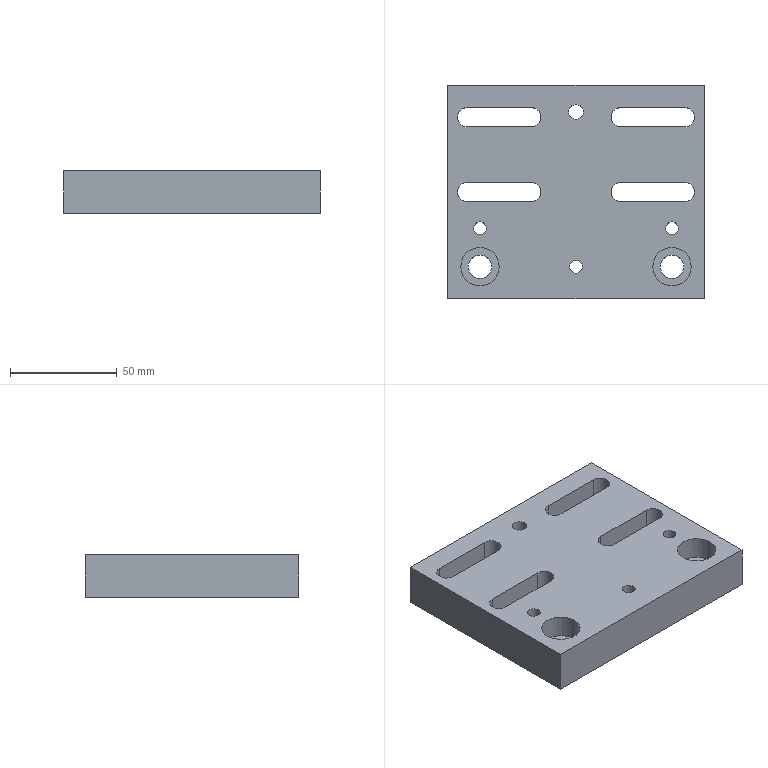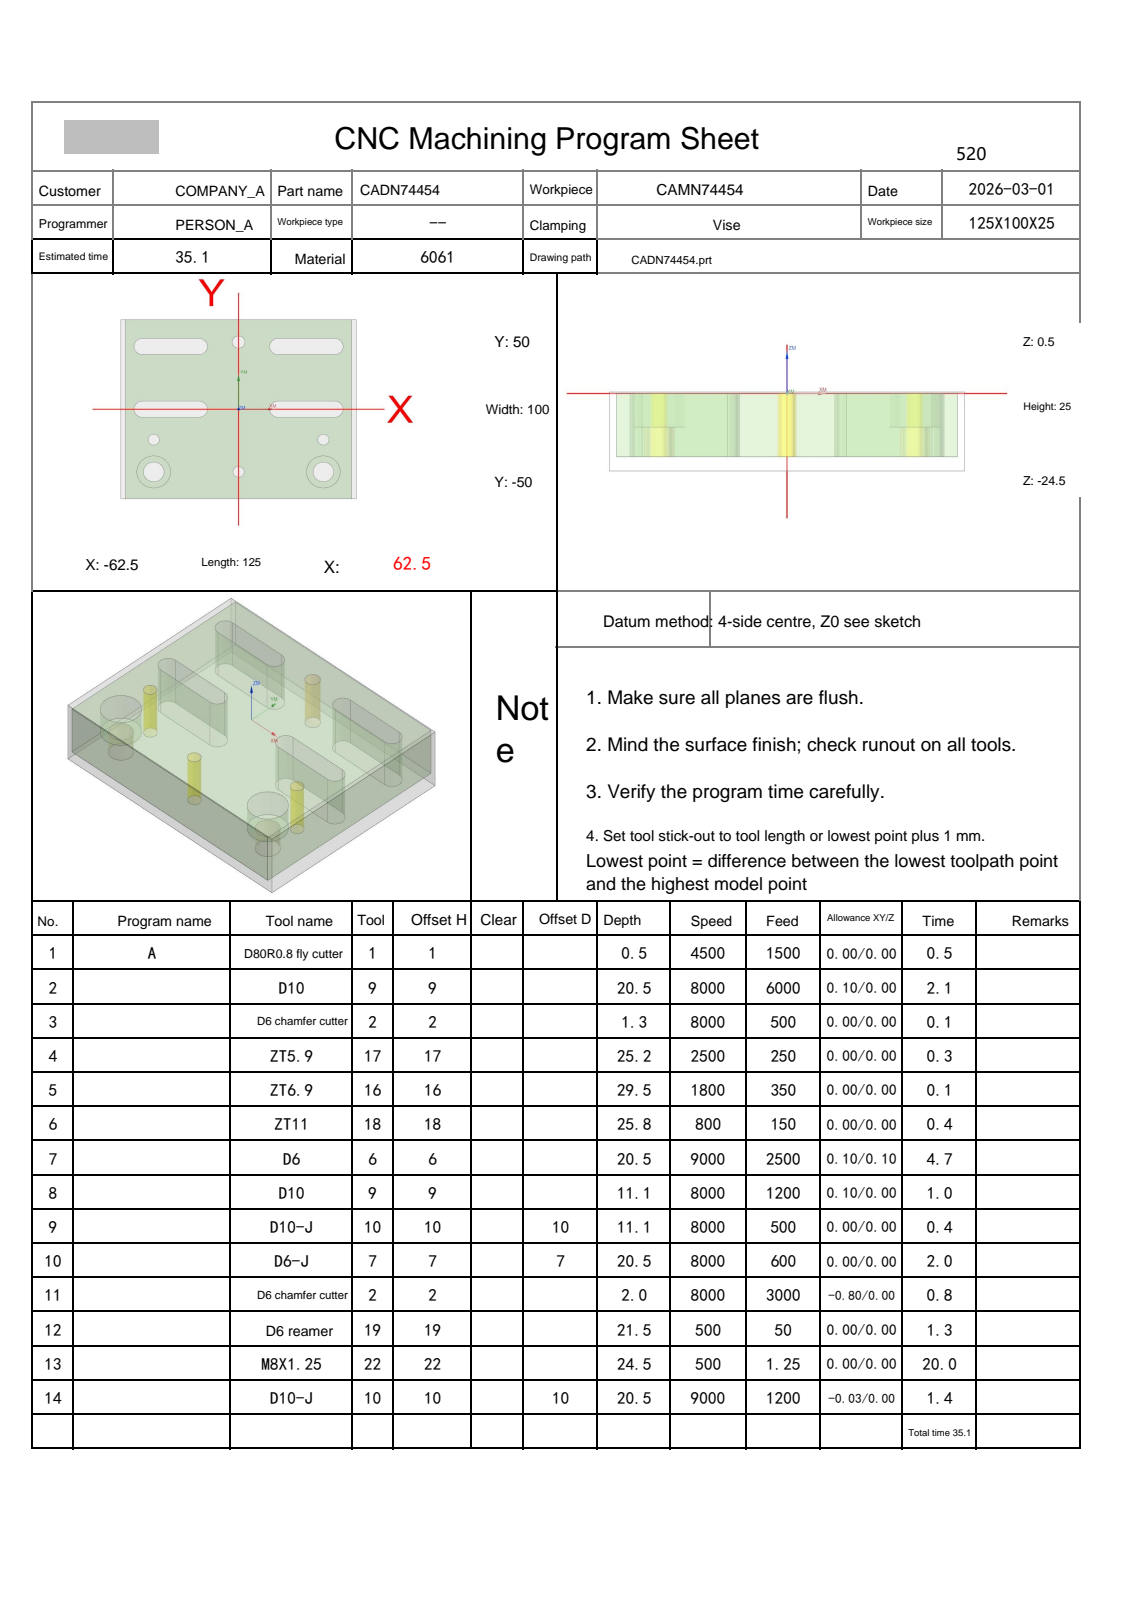NC program | NX | posted by the shop | part box 120 x 100 x 20 mm
Lines 1 to 2069 of 2160, first 1251 of 2067 lines:
%
O0001
(Machine time: 57.03 MIN)
(===Total Tool:11===)
(T1=D80R0.8 fly cutter D=80.  R=0.8  D-  H01 Z=0.    )
(T9=D10     D=10.  R=0.   D-  H09 Z=-20.  )
(T2=D6 chamfer cutter   D=6.   R=0.   D-  H02 Z=-1.5  )
(T17=ZT5.9  D=5.9  DR_a=120 D-  H17 Z=-24.7 )
(T16=ZT6.9  D=6.9  DR_a=120 D-  H16 Z=-29.  )
(T18=ZT11   D=11.  DR_a=118 D-  H18 Z=-25.3 )
(T6=D6      D=6.   R=0.   D-  H06 Z=-20.  )
(T10=D10-J  D=10.  R=0.   D10 H10 Z=-20.  )
(T7=D6-J    D=6.   R=0.   D7  H07 Z=-20.  )
(T19=D6 reamer   D=6.   DR_a=180 D-  H19 Z=-21.  )
(T22=M8X1.25 D=6.8  DR_a=180 D-  H22 Z=-24.  )
G80 G90 G17 G49 G40
G91 G28 Z0
M01
N1 T01 M06
(D80R0.8 fly cutter  D=80. R=0.8 H=01 ce=0.00 di=0.00)
G00 G90 G54 X-105. Y45. M03 S4500
G43 H01 Z50.
M08
Z2.
G01 Z0.0 F1500.
X-100.
X100.
Y0.0
X-100.
Y-45.
X100.
X105.
Z2.
G00 Z50.
G91 G28 Z0.0
M05
M09
G91 G28 Z0.0
M01
N2 T09 M06
(D10  D=10. R=0. H=09 ce=0.10 di=0.00)
G00 G90 G54 X0.0 Y55.1 M03 S8000
G43 H09 Z50.
M08
Z.5
G01 X60. Z.4 F6000.
G02 X65.1 Y50. Z.386 I0.0 J-5.1
G01 Y-50. Z.219
G02 X60. Y-55.1 Z.206 I-5.1 J0.0
G01 X-60. Z.006
G02 X-65.1 Y-50. Z-.008 I0.0 J5.1
G01 Y50. Z-.175
G02 X-60. Y55.1 Z-.188 I5.1 J0.0
G01 X60. Z-.389
G02 X65.1 Y50. Z-.402 I0.0 J-5.1
G01 Y-50. Z-.569
G02 X60. Y-55.1 Z-.582 I-5.1 J0.0
G01 X-60. Z-.783
G02 X-65.1 Y-50. Z-.796 I0.0 J5.1
G01 Y50. Z-.963
G02 X-60. Y55.1 Z-.977 I5.1 J0.0
G01 X60. Z-1.177
G02 X65.1 Y50. Z-1.191 I0.0 J-5.1
G01 Y-50. Z-1.358
G02 X60. Y-55.1 Z-1.371 I-5.1 J0.0
G01 X-60. Z-1.571
G02 X-65.1 Y-50. Z-1.585 I0.0 J5.1
G01 Y50. Z-1.752
G02 X-60. Y55.1 Z-1.765 I5.1 J0.0
G01 X60. Z-1.966
G02 X65.1 Y50. Z-1.979 I0.0 J-5.1
G01 Y-50. Z-2.146
G02 X60. Y-55.1 Z-2.159 I-5.1 J0.0
G01 X-60. Z-2.36
G02 X-65.1 Y-50. Z-2.373 I0.0 J5.1
G01 Y50. Z-2.54
G02 X-60. Y55.1 Z-2.554 I5.1 J0.0
G01 X60. Z-2.754
G02 X65.1 Y50. Z-2.767 I0.0 J-5.1
G01 Y-50. Z-2.934
G02 X60. Y-55.1 Z-2.948 I-5.1 J0.0
G01 X-60. Z-3.148
G02 X-65.1 Y-50. Z-3.162 I0.0 J5.1
G01 Y50. Z-3.329
G02 X-60. Y55.1 Z-3.342 I5.1 J0.0
G01 X60. Z-3.543
G02 X65.1 Y50. Z-3.556 I0.0 J-5.1
G01 Y-50. Z-3.723
G02 X60. Y-55.1 Z-3.736 I-5.1 J0.0
G01 X-60. Z-3.937
G02 X-65.1 Y-50. Z-3.95 I0.0 J5.1
G01 Y50. Z-4.117
G02 X-60. Y55.1 Z-4.131 I5.1 J0.0
G01 X60. Z-4.331
G02 X65.1 Y50. Z-4.344 I0.0 J-5.1
G01 Y-50. Z-4.511
G02 X60. Y-55.1 Z-4.525 I-5.1 J0.0
G01 X-60. Z-4.725
G02 X-65.1 Y-50. Z-4.739 I0.0 J5.1
G01 Y50. Z-4.906
G02 X-60. Y55.1 Z-4.919 I5.1 J0.0
G01 X60. Z-5.119
G02 X65.1 Y50. Z-5.133 I0.0 J-5.1
G01 Y-50. Z-5.3
G02 X60. Y-55.1 Z-5.313 I-5.1 J0.0
G01 X-60. Z-5.514
G02 X-65.1 Y-50. Z-5.527 I0.0 J5.1
G01 Y50. Z-5.694
G02 X-60. Y55.1 Z-5.707 I5.1 J0.0
G01 X60. Z-5.908
G02 X65.1 Y50. Z-5.921 I0.0 J-5.1
G01 Y-50. Z-6.088
G02 X60. Y-55.1 Z-6.102 I-5.1 J0.0
G01 X-60. Z-6.302
G02 X-65.1 Y-50. Z-6.316 I0.0 J5.1
G01 Y50. Z-6.483
G02 X-60. Y55.1 Z-6.496 I5.1 J0.0
G01 X60. Z-6.696
G02 X65.1 Y50. Z-6.71 I0.0 J-5.1
G01 Y-50. Z-6.877
G02 X60. Y-55.1 Z-6.89 I-5.1 J0.0
G01 X-60. Z-7.091
G02 X-65.1 Y-50. Z-7.104 I0.0 J5.1
G01 Y50. Z-7.271
G02 X-60. Y55.1 Z-7.284 I5.1 J0.0
G01 X60. Z-7.485
G02 X65.1 Y50. Z-7.498 I0.0 J-5.1
G01 Y-50. Z-7.665
G02 X60. Y-55.1 Z-7.679 I-5.1 J0.0
G01 X-60. Z-7.879
G02 X-65.1 Y-50. Z-7.892 I0.0 J5.1
G01 Y50. Z-8.059
G02 X-60. Y55.1 Z-8.073 I5.1 J0.0
G01 X60. Z-8.273
G02 X65.1 Y50. Z-8.287 I0.0 J-5.1
G01 Y-50. Z-8.454
G02 X60. Y-55.1 Z-8.467 I-5.1 J0.0
G01 X-60. Z-8.668
G02 X-65.1 Y-50. Z-8.681 I0.0 J5.1
G01 Y50. Z-8.848
G02 X-60. Y55.1 Z-8.861 I5.1 J0.0
G01 X60. Z-9.062
G02 X65.1 Y50. Z-9.075 I0.0 J-5.1
G01 Y-50. Z-9.242
G02 X60. Y-55.1 Z-9.256 I-5.1 J0.0
G01 X-60. Z-9.456
G02 X-65.1 Y-50. Z-9.469 I0.0 J5.1
G01 Y50. Z-9.636
G02 X-60. Y55.1 Z-9.65 I5.1 J0.0
G01 X60. Z-9.85
G02 X65.1 Y50. Z-9.864 I0.0 J-5.1
G01 Y-50. Z-10.031
G02 X60. Y-55.1 Z-10.044 I-5.1 J0.0
G01 X-60. Z-10.244
G02 X-65.1 Y-50. Z-10.258 I0.0 J5.1
G01 Y50. Z-10.425
G02 X-60. Y55.1 Z-10.438 I5.1 J0.0
G01 X60. Z-10.639
G02 X65.1 Y50. Z-10.652 I0.0 J-5.1
G01 Y-50. Z-10.819
G02 X60. Y-55.1 Z-10.832 I-5.1 J0.0
G01 X-60. Z-11.033
G02 X-65.1 Y-50. Z-11.046 I0.0 J5.1
G01 Y50. Z-11.213
G02 X-60. Y55.1 Z-11.227 I5.1 J0.0
G01 X60. Z-11.427
G02 X65.1 Y50. Z-11.441 I0.0 J-5.1
G01 Y-50. Z-11.608
G02 X60. Y-55.1 Z-11.621 I-5.1 J0.0
G01 X-60. Z-11.821
G02 X-65.1 Y-50. Z-11.835 I0.0 J5.1
G01 Y50. Z-12.002
G02 X-60. Y55.1 Z-12.015 I5.1 J0.0
G01 X60. Z-12.216
G02 X65.1 Y50. Z-12.229 I0.0 J-5.1
G01 Y-50. Z-12.396
G02 X60. Y-55.1 Z-12.409 I-5.1 J0.0
G01 X-60. Z-12.61
G02 X-65.1 Y-50. Z-12.623 I0.0 J5.1
G01 Y50. Z-12.79
G02 X-60. Y55.1 Z-12.804 I5.1 J0.0
G01 X60. Z-13.004
G02 X65.1 Y50. Z-13.017 I0.0 J-5.1
G01 Y-50. Z-13.184
G02 X60. Y-55.1 Z-13.198 I-5.1 J0.0
G01 X-60. Z-13.398
G02 X-65.1 Y-50. Z-13.412 I0.0 J5.1
G01 Y50. Z-13.579
G02 X-60. Y55.1 Z-13.592 I5.1 J0.0
G01 X60. Z-13.793
G02 X65.1 Y50. Z-13.806 I0.0 J-5.1
G01 Y-50. Z-13.973
G02 X60. Y-55.1 Z-13.986 I-5.1 J0.0
G01 X-60. Z-14.187
G02 X-65.1 Y-50. Z-14.2 I0.0 J5.1
G01 Y50. Z-14.367
G02 X-60. Y55.1 Z-14.381 I5.1 J0.0
G01 X60. Z-14.581
G02 X65.1 Y50. Z-14.594 I0.0 J-5.1
G01 Y-50. Z-14.761
G02 X60. Y-55.1 Z-14.775 I-5.1 J0.0
G01 X-60. Z-14.975
G02 X-65.1 Y-50. Z-14.989 I0.0 J5.1
G01 Y50. Z-15.156
G02 X-60. Y55.1 Z-15.169 I5.1 J0.0
G01 X60. Z-15.369
G02 X65.1 Y50. Z-15.383 I0.0 J-5.1
G01 Y-50. Z-15.55
G02 X60. Y-55.1 Z-15.563 I-5.1 J0.0
G01 X-60. Z-15.764
G02 X-65.1 Y-50. Z-15.777 I0.0 J5.1
G01 Y50. Z-15.944
G02 X-60. Y55.1 Z-15.957 I5.1 J0.0
G01 X60. Z-16.158
G02 X65.1 Y50. Z-16.171 I0.0 J-5.1
G01 Y-50. Z-16.338
G02 X60. Y-55.1 Z-16.352 I-5.1 J0.0
G01 X-60. Z-16.552
G02 X-65.1 Y-50. Z-16.566 I0.0 J5.1
G01 Y50. Z-16.733
G02 X-60. Y55.1 Z-16.746 I5.1 J0.0
G01 X60. Z-16.946
G02 X65.1 Y50. Z-16.96 I0.0 J-5.1
G01 Y-50. Z-17.127
G02 X60. Y-55.1 Z-17.14 I-5.1 J0.0
G01 X-60. Z-17.341
G02 X-65.1 Y-50. Z-17.354 I0.0 J5.1
G01 Y50. Z-17.521
G02 X-60. Y55.1 Z-17.534 I5.1 J0.0
G01 X60. Z-17.735
G02 X65.1 Y50. Z-17.748 I0.0 J-5.1
G01 Y-50. Z-17.915
G02 X60. Y-55.1 Z-17.929 I-5.1 J0.0
G01 X-60. Z-18.129
G02 X-65.1 Y-50. Z-18.142 I0.0 J5.1
G01 Y50. Z-18.309
G02 X-60. Y55.1 Z-18.323 I5.1 J0.0
G01 X60. Z-18.523
G02 X65.1 Y50. Z-18.537 I0.0 J-5.1
G01 Y-50. Z-18.704
G02 X60. Y-55.1 Z-18.717 I-5.1 J0.0
G01 X-60. Z-18.918
G02 X-65.1 Y-50. Z-18.931 I0.0 J5.1
G01 Y50. Z-19.098
G02 X-60. Y55.1 Z-19.111 I5.1 J0.0
G01 X60. Z-19.312
G02 X65.1 Y50. Z-19.325 I0.0 J-5.1
G01 Y-50. Z-19.492
G02 X60. Y-55.1 Z-19.506 I-5.1 J0.0
G01 X-60. Z-19.706
G02 X-65.1 Y-50. Z-19.719 I0.0 J5.1
G01 Y50. Z-19.886
G02 X-60. Y55.1 Z-19.9 I5.1 J0.0
G01 X0.0 Z-20.
X60.
G02 X65.1 Y50. I0.0 J-5.1
G01 Y-50.
G02 X60. Y-55.1 I-5.1 J0.0
G01 X-60.
G02 X-65.1 Y-50. I0.0 J5.1
G01 Y50.
G02 X-60. Y55.1 I5.1 J0.0
G01 X0.0
X.5
Z-19.
G00 Z50.
G91 G28 Z0.0
M05
M09
G91 G28 Z0.0
M01
N3 T02 M06
(D6 chamfer cutter  D=6. R=0. H=02 ce=0.00 di=0.00)
G00 G90 G54 X45. Y-17. M03 S8000
G43 H02 Z50.
M08
G98 G81 X45. Y-17. Z-.8 R1. F500.
Y-35.
X0.0
X-45.
Y-17.
X0.0 Y37.5
G80
G00 Z50.
G91 G28 Z0.0
M05
M09
G91 G28 Z0.0
M01
N4 T17 M06
(ZT5.9 D=5.9 DR_a=120 H=17)
G00 G90 G54 X45. Y-17. M03 S2500
G43 H17 Z50.
M08
G98 G83 X45. Y-17. Z-24.703 R1. F250. Q2.
X0.0 Y-35.
X-45. Y-17.
G80
G00 Z50.
G91 G28 Z0.0
M05
M09
G91 G28 Z0.0
M01
N5 T16 M06
(ZT6.9 D=6.9 DR_a=120 H=16)
G00 G90 G54 X0.0 Y37.5 M03 S1800
G43 H16 Z50.
M08
G98 G83 X0.0 Y37.5 Z-29. R1. F350. Q3.
G80
G00 Z50.
G91 G28 Z0.0
M05
M09
G91 G28 Z0.0
M01
N6 T18 M06
(ZT11 D=11. DR_a=118 H=18)
G00 G90 G54 X-45. Y-35. M03 S800
G43 H18 Z50.
M08
G98 G83 X-45. Y-35. Z-25.305 R1. F150. Q2.
X45.
G80
G00 Z50.
G91 G28 Z0.0
M05
M09
G91 G28 Z0.0
M01
N7 T06 M06
(D6  D=6. R=0. H=06 ce=0.10 di=0.10)
G00 G90 G54 X36. Y36.4 M03 S9000
G43 H06 Z50.
M08
Z.5
G01 X21. Z.391 F2500.
G03 X19.6 Y35. Z.375 I0.0 J-1.4
X21. Y33.6 Z.359 I1.4 J0.0
G01 X51. Z.141
G03 X52.4 Y35. Z.125 I0.0 J1.4
X51. Y36.4 Z.109 I-1.4 J0.0
G01 X21. Z-.109
G03 X19.6 Y35. Z-.125 I0.0 J-1.4
X21. Y33.6 Z-.141 I1.4 J0.0
G01 X51. Z-.359
G03 X52.4 Y35. Z-.375 I0.0 J1.4
X51. Y36.4 Z-.391 I-1.4 J0.0
G01 X21. Z-.609
G03 X19.6 Y35. Z-.625 I0.0 J-1.4
X21. Y33.6 Z-.641 I1.4 J0.0
G01 X51. Z-.859
G03 X52.4 Y35. Z-.875 I0.0 J1.4
X51. Y36.4 Z-.891 I-1.4 J0.0
G01 X21. Z-1.109
G03 X19.6 Y35. Z-1.125 I0.0 J-1.4
X21. Y33.6 Z-1.141 I1.4 J0.0
G01 X51. Z-1.359
G03 X52.4 Y35. Z-1.375 I0.0 J1.4
X51. Y36.4 Z-1.391 I-1.4 J0.0
G01 X21. Z-1.609
G03 X19.6 Y35. Z-1.625 I0.0 J-1.4
X21. Y33.6 Z-1.641 I1.4 J0.0
G01 X51. Z-1.859
G03 X52.4 Y35. Z-1.875 I0.0 J1.4
X51. Y36.4 Z-1.891 I-1.4 J0.0
G01 X21. Z-2.109
G03 X19.6 Y35. Z-2.125 I0.0 J-1.4
X21. Y33.6 Z-2.141 I1.4 J0.0
G01 X51. Z-2.359
G03 X52.4 Y35. Z-2.375 I0.0 J1.4
X51. Y36.4 Z-2.391 I-1.4 J0.0
G01 X21. Z-2.609
G03 X19.6 Y35. Z-2.625 I0.0 J-1.4
X21. Y33.6 Z-2.641 I1.4 J0.0
G01 X51. Z-2.859
G03 X52.4 Y35. Z-2.875 I0.0 J1.4
X51. Y36.4 Z-2.891 I-1.4 J0.0
G01 X21. Z-3.109
G03 X19.6 Y35. Z-3.125 I0.0 J-1.4
X21. Y33.6 Z-3.141 I1.4 J0.0
G01 X51. Z-3.359
G03 X52.4 Y35. Z-3.375 I0.0 J1.4
X51. Y36.4 Z-3.391 I-1.4 J0.0
G01 X21. Z-3.609
G03 X19.6 Y35. Z-3.625 I0.0 J-1.4
X21. Y33.6 Z-3.641 I1.4 J0.0
G01 X51. Z-3.859
G03 X52.4 Y35. Z-3.875 I0.0 J1.4
X51. Y36.4 Z-3.891 I-1.4 J0.0
G01 X21. Z-4.109
G03 X19.6 Y35. Z-4.125 I0.0 J-1.4
X21. Y33.6 Z-4.141 I1.4 J0.0
G01 X51. Z-4.359
G03 X52.4 Y35. Z-4.375 I0.0 J1.4
X51. Y36.4 Z-4.391 I-1.4 J0.0
G01 X21. Z-4.609
G03 X19.6 Y35. Z-4.625 I0.0 J-1.4
X21. Y33.6 Z-4.641 I1.4 J0.0
G01 X51. Z-4.859
G03 X52.4 Y35. Z-4.875 I0.0 J1.4
X51. Y36.4 Z-4.891 I-1.4 J0.0
G01 X21. Z-5.109
G03 X19.6 Y35. Z-5.125 I0.0 J-1.4
X21. Y33.6 Z-5.141 I1.4 J0.0
G01 X51. Z-5.359
G03 X52.4 Y35. Z-5.375 I0.0 J1.4
X51. Y36.4 Z-5.391 I-1.4 J0.0
G01 X21. Z-5.609
G03 X19.6 Y35. Z-5.625 I0.0 J-1.4
X21. Y33.6 Z-5.641 I1.4 J0.0
G01 X51. Z-5.859
G03 X52.4 Y35. Z-5.875 I0.0 J1.4
X51. Y36.4 Z-5.891 I-1.4 J0.0
G01 X21. Z-6.109
G03 X19.6 Y35. Z-6.125 I0.0 J-1.4
X21. Y33.6 Z-6.141 I1.4 J0.0
G01 X51. Z-6.359
G03 X52.4 Y35. Z-6.375 I0.0 J1.4
X51. Y36.4 Z-6.391 I-1.4 J0.0
G01 X21. Z-6.609
G03 X19.6 Y35. Z-6.625 I0.0 J-1.4
X21. Y33.6 Z-6.641 I1.4 J0.0
G01 X51. Z-6.859
G03 X52.4 Y35. Z-6.875 I0.0 J1.4
X51. Y36.4 Z-6.891 I-1.4 J0.0
G01 X21. Z-7.109
G03 X19.6 Y35. Z-7.125 I0.0 J-1.4
X21. Y33.6 Z-7.141 I1.4 J0.0
G01 X51. Z-7.359
G03 X52.4 Y35. Z-7.375 I0.0 J1.4
X51. Y36.4 Z-7.391 I-1.4 J0.0
G01 X21. Z-7.609
G03 X19.6 Y35. Z-7.625 I0.0 J-1.4
X21. Y33.6 Z-7.641 I1.4 J0.0
G01 X51. Z-7.859
G03 X52.4 Y35. Z-7.875 I0.0 J1.4
X51. Y36.4 Z-7.891 I-1.4 J0.0
G01 X21. Z-8.109
G03 X19.6 Y35. Z-8.125 I0.0 J-1.4
X21. Y33.6 Z-8.141 I1.4 J0.0
G01 X51. Z-8.359
G03 X52.4 Y35. Z-8.375 I0.0 J1.4
X51. Y36.4 Z-8.391 I-1.4 J0.0
G01 X21. Z-8.609
G03 X19.6 Y35. Z-8.625 I0.0 J-1.4
X21. Y33.6 Z-8.641 I1.4 J0.0
G01 X51. Z-8.859
G03 X52.4 Y35. Z-8.875 I0.0 J1.4
X51. Y36.4 Z-8.891 I-1.4 J0.0
G01 X21. Z-9.109
G03 X19.6 Y35. Z-9.125 I0.0 J-1.4
X21. Y33.6 Z-9.141 I1.4 J0.0
G01 X51. Z-9.359
G03 X52.4 Y35. Z-9.375 I0.0 J1.4
X51. Y36.4 Z-9.391 I-1.4 J0.0
G01 X21. Z-9.609
G03 X19.6 Y35. Z-9.625 I0.0 J-1.4
X21. Y33.6 Z-9.641 I1.4 J0.0
G01 X51. Z-9.859
G03 X52.4 Y35. Z-9.875 I0.0 J1.4
X51. Y36.4 Z-9.891 I-1.4 J0.0
G01 X21. Z-10.109
G03 X19.6 Y35. Z-10.125 I0.0 J-1.4
X21. Y33.6 Z-10.141 I1.4 J0.0
G01 X51. Z-10.359
G03 X52.4 Y35. Z-10.375 I0.0 J1.4
X51. Y36.4 Z-10.391 I-1.4 J0.0
G01 X21. Z-10.609
G03 X19.6 Y35. Z-10.625 I0.0 J-1.4
X21. Y33.6 Z-10.641 I1.4 J0.0
G01 X51. Z-10.859
G03 X52.4 Y35. Z-10.875 I0.0 J1.4
X51. Y36.4 Z-10.891 I-1.4 J0.0
G01 X21. Z-11.109
G03 X19.6 Y35. Z-11.125 I0.0 J-1.4
X21. Y33.6 Z-11.141 I1.4 J0.0
G01 X51. Z-11.359
G03 X52.4 Y35. Z-11.375 I0.0 J1.4
X51. Y36.4 Z-11.391 I-1.4 J0.0
G01 X21. Z-11.609
G03 X19.6 Y35. Z-11.625 I0.0 J-1.4
X21. Y33.6 Z-11.641 I1.4 J0.0
G01 X51. Z-11.859
G03 X52.4 Y35. Z-11.875 I0.0 J1.4
X51. Y36.4 Z-11.891 I-1.4 J0.0
G01 X21. Z-12.109
G03 X19.6 Y35. Z-12.125 I0.0 J-1.4
X21. Y33.6 Z-12.141 I1.4 J0.0
G01 X51. Z-12.359
G03 X52.4 Y35. Z-12.375 I0.0 J1.4
X51. Y36.4 Z-12.391 I-1.4 J0.0
G01 X21. Z-12.609
G03 X19.6 Y35. Z-12.625 I0.0 J-1.4
X21. Y33.6 Z-12.641 I1.4 J0.0
G01 X51. Z-12.859
G03 X52.4 Y35. Z-12.875 I0.0 J1.4
X51. Y36.4 Z-12.891 I-1.4 J0.0
G01 X21. Z-13.109
G03 X19.6 Y35. Z-13.125 I0.0 J-1.4
X21. Y33.6 Z-13.141 I1.4 J0.0
G01 X51. Z-13.359
G03 X52.4 Y35. Z-13.375 I0.0 J1.4
X51. Y36.4 Z-13.391 I-1.4 J0.0
G01 X21. Z-13.609
G03 X19.6 Y35. Z-13.625 I0.0 J-1.4
X21. Y33.6 Z-13.641 I1.4 J0.0
G01 X51. Z-13.859
G03 X52.4 Y35. Z-13.875 I0.0 J1.4
X51. Y36.4 Z-13.891 I-1.4 J0.0
G01 X21. Z-14.109
G03 X19.6 Y35. Z-14.125 I0.0 J-1.4
X21. Y33.6 Z-14.141 I1.4 J0.0
G01 X51. Z-14.359
G03 X52.4 Y35. Z-14.375 I0.0 J1.4
X51. Y36.4 Z-14.391 I-1.4 J0.0
G01 X21. Z-14.609
G03 X19.6 Y35. Z-14.625 I0.0 J-1.4
X21. Y33.6 Z-14.641 I1.4 J0.0
G01 X51. Z-14.859
G03 X52.4 Y35. Z-14.875 I0.0 J1.4
X51. Y36.4 Z-14.891 I-1.4 J0.0
G01 X21. Z-15.109
G03 X19.6 Y35. Z-15.125 I0.0 J-1.4
X21. Y33.6 Z-15.141 I1.4 J0.0
G01 X51. Z-15.359
G03 X52.4 Y35. Z-15.375 I0.0 J1.4
X51. Y36.4 Z-15.391 I-1.4 J0.0
G01 X21. Z-15.609
G03 X19.6 Y35. Z-15.625 I0.0 J-1.4
X21. Y33.6 Z-15.641 I1.4 J0.0
G01 X51. Z-15.859
G03 X52.4 Y35. Z-15.875 I0.0 J1.4
X51. Y36.4 Z-15.891 I-1.4 J0.0
G01 X21. Z-16.109
G03 X19.6 Y35. Z-16.125 I0.0 J-1.4
X21. Y33.6 Z-16.141 I1.4 J0.0
G01 X51. Z-16.359
G03 X52.4 Y35. Z-16.375 I0.0 J1.4
X51. Y36.4 Z-16.391 I-1.4 J0.0
G01 X21. Z-16.609
G03 X19.6 Y35. Z-16.625 I0.0 J-1.4
X21. Y33.6 Z-16.641 I1.4 J0.0
G01 X51. Z-16.859
G03 X52.4 Y35. Z-16.875 I0.0 J1.4
X51. Y36.4 Z-16.891 I-1.4 J0.0
G01 X21. Z-17.109
G03 X19.6 Y35. Z-17.125 I0.0 J-1.4
X21. Y33.6 Z-17.141 I1.4 J0.0
G01 X51. Z-17.359
G03 X52.4 Y35. Z-17.375 I0.0 J1.4
X51. Y36.4 Z-17.391 I-1.4 J0.0
G01 X21. Z-17.609
G03 X19.6 Y35. Z-17.625 I0.0 J-1.4
X21. Y33.6 Z-17.641 I1.4 J0.0
G01 X51. Z-17.859
G03 X52.4 Y35. Z-17.875 I0.0 J1.4
X51. Y36.4 Z-17.891 I-1.4 J0.0
G01 X21. Z-18.109
G03 X19.6 Y35. Z-18.125 I0.0 J-1.4
X21. Y33.6 Z-18.141 I1.4 J0.0
G01 X51. Z-18.359
G03 X52.4 Y35. Z-18.375 I0.0 J1.4
X51. Y36.4 Z-18.391 I-1.4 J0.0
G01 X21. Z-18.609
G03 X19.6 Y35. Z-18.625 I0.0 J-1.4
X21. Y33.6 Z-18.641 I1.4 J0.0
G01 X51. Z-18.859
G03 X52.4 Y35. Z-18.875 I0.0 J1.4
X51. Y36.4 Z-18.891 I-1.4 J0.0
G01 X21. Z-19.109
G03 X19.6 Y35. Z-19.125 I0.0 J-1.4
X21. Y33.6 Z-19.141 I1.4 J0.0
G01 X51. Z-19.359
G03 X52.4 Y35. Z-19.375 I0.0 J1.4
X51. Y36.4 Z-19.391 I-1.4 J0.0
G01 X21. Z-19.609
G03 X19.6 Y35. Z-19.625 I0.0 J-1.4
X21. Y33.6 Z-19.641 I1.4 J0.0
G01 X51. Z-19.859
G03 X52.4 Y35. Z-19.875 I0.0 J1.4
X51. Y36.4 Z-19.891 I-1.4 J0.0
G01 X36. Z-20.
X21.
G03 X19.6 Y35. I0.0 J-1.4
X21. Y33.6 I1.4 J0.0
G01 X51.
G03 X52.4 Y35. I0.0 J1.4
X51. Y36.4 I-1.4 J0.0
G01 X36.
X35.5
Z-19.
G00 Z50.
X36. Y1.4
Z.5
G01 X21. Z.391
G03 X19.6 Y0.0 Z.375 I0.0 J-1.4
X21. Y-1.4 Z.359 I1.4 J0.0
G01 X51. Z.141
G03 X52.4 Y0.0 Z.125 I0.0 J1.4
X51. Y1.4 Z.109 I-1.4 J0.0
G01 X21. Z-.109
G03 X19.6 Y0.0 Z-.125 I0.0 J-1.4
X21. Y-1.4 Z-.141 I1.4 J0.0
G01 X51. Z-.359
G03 X52.4 Y0.0 Z-.375 I0.0 J1.4
X51. Y1.4 Z-.391 I-1.4 J0.0
G01 X21. Z-.609
G03 X19.6 Y0.0 Z-.625 I0.0 J-1.4
X21. Y-1.4 Z-.641 I1.4 J0.0
G01 X51. Z-.859
G03 X52.4 Y0.0 Z-.875 I0.0 J1.4
X51. Y1.4 Z-.891 I-1.4 J0.0
G01 X21. Z-1.109
G03 X19.6 Y0.0 Z-1.125 I0.0 J-1.4
X21. Y-1.4 Z-1.141 I1.4 J0.0
G01 X51. Z-1.359
G03 X52.4 Y0.0 Z-1.375 I0.0 J1.4
X51. Y1.4 Z-1.391 I-1.4 J0.0
G01 X21. Z-1.609
G03 X19.6 Y0.0 Z-1.625 I0.0 J-1.4
X21. Y-1.4 Z-1.641 I1.4 J0.0
G01 X51. Z-1.859
G03 X52.4 Y0.0 Z-1.875 I0.0 J1.4
X51. Y1.4 Z-1.891 I-1.4 J0.0
G01 X21. Z-2.109
G03 X19.6 Y0.0 Z-2.125 I0.0 J-1.4
X21. Y-1.4 Z-2.141 I1.4 J0.0
G01 X51. Z-2.359
G03 X52.4 Y0.0 Z-2.375 I0.0 J1.4
X51. Y1.4 Z-2.391 I-1.4 J0.0
G01 X21. Z-2.609
G03 X19.6 Y0.0 Z-2.625 I0.0 J-1.4
X21. Y-1.4 Z-2.641 I1.4 J0.0
G01 X51. Z-2.859
G03 X52.4 Y0.0 Z-2.875 I0.0 J1.4
X51. Y1.4 Z-2.891 I-1.4 J0.0
G01 X21. Z-3.109
G03 X19.6 Y0.0 Z-3.125 I0.0 J-1.4
X21. Y-1.4 Z-3.141 I1.4 J0.0
G01 X51. Z-3.359
G03 X52.4 Y0.0 Z-3.375 I0.0 J1.4
X51. Y1.4 Z-3.391 I-1.4 J0.0
G01 X21. Z-3.609
G03 X19.6 Y0.0 Z-3.625 I0.0 J-1.4
X21. Y-1.4 Z-3.641 I1.4 J0.0
G01 X51. Z-3.859
G03 X52.4 Y0.0 Z-3.875 I0.0 J1.4
X51. Y1.4 Z-3.891 I-1.4 J0.0
G01 X21. Z-4.109
G03 X19.6 Y0.0 Z-4.125 I0.0 J-1.4
X21. Y-1.4 Z-4.141 I1.4 J0.0
G01 X51. Z-4.359
G03 X52.4 Y0.0 Z-4.375 I0.0 J1.4
X51. Y1.4 Z-4.391 I-1.4 J0.0
G01 X21. Z-4.609
G03 X19.6 Y0.0 Z-4.625 I0.0 J-1.4
X21. Y-1.4 Z-4.641 I1.4 J0.0
G01 X51. Z-4.859
G03 X52.4 Y0.0 Z-4.875 I0.0 J1.4
X51. Y1.4 Z-4.891 I-1.4 J0.0
G01 X21. Z-5.109
G03 X19.6 Y0.0 Z-5.125 I0.0 J-1.4
X21. Y-1.4 Z-5.141 I1.4 J0.0
G01 X51. Z-5.359
G03 X52.4 Y0.0 Z-5.375 I0.0 J1.4
X51. Y1.4 Z-5.391 I-1.4 J0.0
G01 X21. Z-5.609
G03 X19.6 Y0.0 Z-5.625 I0.0 J-1.4
X21. Y-1.4 Z-5.641 I1.4 J0.0
G01 X51. Z-5.859
G03 X52.4 Y0.0 Z-5.875 I0.0 J1.4
X51. Y1.4 Z-5.891 I-1.4 J0.0
G01 X21. Z-6.109
G03 X19.6 Y0.0 Z-6.125 I0.0 J-1.4
X21. Y-1.4 Z-6.141 I1.4 J0.0
G01 X51. Z-6.359
G03 X52.4 Y0.0 Z-6.375 I0.0 J1.4
X51. Y1.4 Z-6.391 I-1.4 J0.0
G01 X21. Z-6.609
G03 X19.6 Y0.0 Z-6.625 I0.0 J-1.4
X21. Y-1.4 Z-6.641 I1.4 J0.0
G01 X51. Z-6.859
G03 X52.4 Y0.0 Z-6.875 I0.0 J1.4
X51. Y1.4 Z-6.891 I-1.4 J0.0
G01 X21. Z-7.109
G03 X19.6 Y0.0 Z-7.125 I0.0 J-1.4
X21. Y-1.4 Z-7.141 I1.4 J0.0
G01 X51. Z-7.359
G03 X52.4 Y0.0 Z-7.375 I0.0 J1.4
X51. Y1.4 Z-7.391 I-1.4 J0.0
G01 X21. Z-7.609
G03 X19.6 Y0.0 Z-7.625 I0.0 J-1.4
X21. Y-1.4 Z-7.641 I1.4 J0.0
G01 X51. Z-7.859
G03 X52.4 Y0.0 Z-7.875 I0.0 J1.4
X51. Y1.4 Z-7.891 I-1.4 J0.0
G01 X21. Z-8.109
G03 X19.6 Y0.0 Z-8.125 I0.0 J-1.4
X21. Y-1.4 Z-8.141 I1.4 J0.0
G01 X51. Z-8.359
G03 X52.4 Y0.0 Z-8.375 I0.0 J1.4
X51. Y1.4 Z-8.391 I-1.4 J0.0
G01 X21. Z-8.609
G03 X19.6 Y0.0 Z-8.625 I0.0 J-1.4
X21. Y-1.4 Z-8.641 I1.4 J0.0
G01 X51. Z-8.859
G03 X52.4 Y0.0 Z-8.875 I0.0 J1.4
X51. Y1.4 Z-8.891 I-1.4 J0.0
G01 X21. Z-9.109
G03 X19.6 Y0.0 Z-9.125 I0.0 J-1.4
X21. Y-1.4 Z-9.141 I1.4 J0.0
G01 X51. Z-9.359
G03 X52.4 Y0.0 Z-9.375 I0.0 J1.4
X51. Y1.4 Z-9.391 I-1.4 J0.0
G01 X21. Z-9.609
G03 X19.6 Y0.0 Z-9.625 I0.0 J-1.4
X21. Y-1.4 Z-9.641 I1.4 J0.0
G01 X51. Z-9.859
G03 X52.4 Y0.0 Z-9.875 I0.0 J1.4
X51. Y1.4 Z-9.891 I-1.4 J0.0
G01 X21. Z-10.109
G03 X19.6 Y0.0 Z-10.125 I0.0 J-1.4
X21. Y-1.4 Z-10.141 I1.4 J0.0
G01 X51. Z-10.359
G03 X52.4 Y0.0 Z-10.375 I0.0 J1.4
X51. Y1.4 Z-10.391 I-1.4 J0.0
G01 X21. Z-10.609
G03 X19.6 Y0.0 Z-10.625 I0.0 J-1.4
X21. Y-1.4 Z-10.641 I1.4 J0.0
G01 X51. Z-10.859
G03 X52.4 Y0.0 Z-10.875 I0.0 J1.4
X51. Y1.4 Z-10.891 I-1.4 J0.0
G01 X21. Z-11.109
G03 X19.6 Y0.0 Z-11.125 I0.0 J-1.4
X21. Y-1.4 Z-11.141 I1.4 J0.0
G01 X51. Z-11.359
G03 X52.4 Y0.0 Z-11.375 I0.0 J1.4
X51. Y1.4 Z-11.391 I-1.4 J0.0
G01 X21. Z-11.609
G03 X19.6 Y0.0 Z-11.625 I0.0 J-1.4
X21. Y-1.4 Z-11.641 I1.4 J0.0
G01 X51. Z-11.859
G03 X52.4 Y0.0 Z-11.875 I0.0 J1.4
X51. Y1.4 Z-11.891 I-1.4 J0.0
G01 X21. Z-12.109
G03 X19.6 Y0.0 Z-12.125 I0.0 J-1.4
X21. Y-1.4 Z-12.141 I1.4 J0.0
G01 X51. Z-12.359
G03 X52.4 Y0.0 Z-12.375 I0.0 J1.4
X51. Y1.4 Z-12.391 I-1.4 J0.0
G01 X21. Z-12.609
G03 X19.6 Y0.0 Z-12.625 I0.0 J-1.4
X21. Y-1.4 Z-12.641 I1.4 J0.0
G01 X51. Z-12.859
G03 X52.4 Y0.0 Z-12.875 I0.0 J1.4
X51. Y1.4 Z-12.891 I-1.4 J0.0
G01 X21. Z-13.109
G03 X19.6 Y0.0 Z-13.125 I0.0 J-1.4
X21. Y-1.4 Z-13.141 I1.4 J0.0
G01 X51. Z-13.359
G03 X52.4 Y0.0 Z-13.375 I0.0 J1.4
X51. Y1.4 Z-13.391 I-1.4 J0.0
G01 X21. Z-13.609
G03 X19.6 Y0.0 Z-13.625 I0.0 J-1.4
X21. Y-1.4 Z-13.641 I1.4 J0.0
G01 X51. Z-13.859
G03 X52.4 Y0.0 Z-13.875 I0.0 J1.4
X51. Y1.4 Z-13.891 I-1.4 J0.0
G01 X21. Z-14.109
G03 X19.6 Y0.0 Z-14.125 I0.0 J-1.4
X21. Y-1.4 Z-14.141 I1.4 J0.0
G01 X51. Z-14.359
G03 X52.4 Y0.0 Z-14.375 I0.0 J1.4
X51. Y1.4 Z-14.391 I-1.4 J0.0
G01 X21. Z-14.609
G03 X19.6 Y0.0 Z-14.625 I0.0 J-1.4
X21. Y-1.4 Z-14.641 I1.4 J0.0
G01 X51. Z-14.859
G03 X52.4 Y0.0 Z-14.875 I0.0 J1.4
X51. Y1.4 Z-14.891 I-1.4 J0.0
G01 X21. Z-15.109
G03 X19.6 Y0.0 Z-15.125 I0.0 J-1.4
X21. Y-1.4 Z-15.141 I1.4 J0.0
G01 X51. Z-15.359
G03 X52.4 Y0.0 Z-15.375 I0.0 J1.4
X51. Y1.4 Z-15.391 I-1.4 J0.0
G01 X21. Z-15.609
G03 X19.6 Y0.0 Z-15.625 I0.0 J-1.4
X21. Y-1.4 Z-15.641 I1.4 J0.0
G01 X51. Z-15.859
G03 X52.4 Y0.0 Z-15.875 I0.0 J1.4
X51. Y1.4 Z-15.891 I-1.4 J0.0
G01 X21. Z-16.109
G03 X19.6 Y0.0 Z-16.125 I0.0 J-1.4
X21. Y-1.4 Z-16.141 I1.4 J0.0
G01 X51. Z-16.359
G03 X52.4 Y0.0 Z-16.375 I0.0 J1.4
X51. Y1.4 Z-16.391 I-1.4 J0.0
G01 X21. Z-16.609
G03 X19.6 Y0.0 Z-16.625 I0.0 J-1.4
X21. Y-1.4 Z-16.641 I1.4 J0.0
G01 X51. Z-16.859
G03 X52.4 Y0.0 Z-16.875 I0.0 J1.4
X51. Y1.4 Z-16.891 I-1.4 J0.0
G01 X21. Z-17.109
G03 X19.6 Y0.0 Z-17.125 I0.0 J-1.4
X21. Y-1.4 Z-17.141 I1.4 J0.0
G01 X51. Z-17.359
G03 X52.4 Y0.0 Z-17.375 I0.0 J1.4
X51. Y1.4 Z-17.391 I-1.4 J0.0
G01 X21. Z-17.609
G03 X19.6 Y0.0 Z-17.625 I0.0 J-1.4
X21. Y-1.4 Z-17.641 I1.4 J0.0
G01 X51. Z-17.859
G03 X52.4 Y0.0 Z-17.875 I0.0 J1.4
X51. Y1.4 Z-17.891 I-1.4 J0.0
G01 X21. Z-18.109
G03 X19.6 Y0.0 Z-18.125 I0.0 J-1.4
X21. Y-1.4 Z-18.141 I1.4 J0.0
G01 X51. Z-18.359
G03 X52.4 Y0.0 Z-18.375 I0.0 J1.4
X51. Y1.4 Z-18.391 I-1.4 J0.0
G01 X21. Z-18.609
G03 X19.6 Y0.0 Z-18.625 I0.0 J-1.4
X21. Y-1.4 Z-18.641 I1.4 J0.0
G01 X51. Z-18.859
G03 X52.4 Y0.0 Z-18.875 I0.0 J1.4
X51. Y1.4 Z-18.891 I-1.4 J0.0
G01 X21. Z-19.109
G03 X19.6 Y0.0 Z-19.125 I0.0 J-1.4
X21. Y-1.4 Z-19.141 I1.4 J0.0
G01 X51. Z-19.359
G03 X52.4 Y0.0 Z-19.375 I0.0 J1.4
X51. Y1.4 Z-19.391 I-1.4 J0.0
G01 X21. Z-19.609
G03 X19.6 Y0.0 Z-19.625 I0.0 J-1.4
X21. Y-1.4 Z-19.641 I1.4 J0.0
G01 X51. Z-19.859
G03 X52.4 Y0.0 Z-19.875 I0.0 J1.4
X51. Y1.4 Z-19.891 I-1.4 J0.0
G01 X36. Z-20.
X21.
G03 X19.6 Y0.0 I0.0 J-1.4
X21. Y-1.4 I1.4 J0.0
G01 X51.
G03 X52.4 Y0.0 I0.0 J1.4
X51. Y1.4 I-1.4 J0.0
G01 X36.
X35.5
Z-19.
G00 Z50.
X-36.
Z.5
G01 X-51. Z.391
G03 X-52.4 Y0.0 Z.375 I0.0 J-1.4
X-51. Y-1.4 Z.359 I1.4 J0.0
G01 X-21. Z.141
G03 X-19.6 Y0.0 Z.125 I0.0 J1.4
X-21. Y1.4 Z.109 I-1.4 J0.0
G01 X-51. Z-.109
G03 X-52.4 Y0.0 Z-.125 I0.0 J-1.4
X-51. Y-1.4 Z-.141 I1.4 J0.0
G01 X-21. Z-.359
G03 X-19.6 Y0.0 Z-.375 I0.0 J1.4
X-21. Y1.4 Z-.391 I-1.4 J0.0
G01 X-51. Z-.609
G03 X-52.4 Y0.0 Z-.625 I0.0 J-1.4
X-51. Y-1.4 Z-.641 I1.4 J0.0
G01 X-21. Z-.859
G03 X-19.6 Y0.0 Z-.875 I0.0 J1.4
X-21. Y1.4 Z-.891 I-1.4 J0.0
G01 X-51. Z-1.109
G03 X-52.4 Y0.0 Z-1.125 I0.0 J-1.4
X-51. Y-1.4 Z-1.141 I1.4 J0.0
G01 X-21. Z-1.359
G03 X-19.6 Y0.0 Z-1.375 I0.0 J1.4
X-21. Y1.4 Z-1.391 I-1.4 J0.0
G01 X-51. Z-1.609
G03 X-52.4 Y0.0 Z-1.625 I0.0 J-1.4
X-51. Y-1.4 Z-1.641 I1.4 J0.0
G01 X-21. Z-1.859
G03 X-19.6 Y0.0 Z-1.875 I0.0 J1.4
X-21. Y1.4 Z-1.891 I-1.4 J0.0
G01 X-51. Z-2.109
G03 X-52.4 Y0.0 Z-2.125 I0.0 J-1.4
X-51. Y-1.4 Z-2.141 I1.4 J0.0
G01 X-21. Z-2.359
G03 X-19.6 Y0.0 Z-2.375 I0.0 J1.4
X-21. Y1.4 Z-2.391 I-1.4 J0.0
G01 X-51. Z-2.609
G03 X-52.4 Y0.0 Z-2.625 I0.0 J-1.4
X-51. Y-1.4 Z-2.641 I1.4 J0.0
G01 X-21. Z-2.859
G03 X-19.6 Y0.0 Z-2.875 I0.0 J1.4
X-21. Y1.4 Z-2.891 I-1.4 J0.0
G01 X-51. Z-3.109
G03 X-52.4 Y0.0 Z-3.125 I0.0 J-1.4
X-51. Y-1.4 Z-3.141 I1.4 J0.0
G01 X-21. Z-3.359
G03 X-19.6 Y0.0 Z-3.375 I0.0 J1.4
X-21. Y1.4 Z-3.391 I-1.4 J0.0
G01 X-51. Z-3.609
G03 X-52.4 Y0.0 Z-3.625 I0.0 J-1.4
X-51. Y-1.4 Z-3.641 I1.4 J0.0
G01 X-21. Z-3.859
G03 X-19.6 Y0.0 Z-3.875 I0.0 J1.4
X-21. Y1.4 Z-3.891 I-1.4 J0.0
G01 X-51. Z-4.109
G03 X-52.4 Y0.0 Z-4.125 I0.0 J-1.4
X-51. Y-1.4 Z-4.141 I1.4 J0.0
G01 X-21. Z-4.359
G03 X-19.6 Y0.0 Z-4.375 I0.0 J1.4
X-21. Y1.4 Z-4.391 I-1.4 J0.0
G01 X-51. Z-4.609
G03 X-52.4 Y0.0 Z-4.625 I0.0 J-1.4
X-51. Y-1.4 Z-4.641 I1.4 J0.0
G01 X-21. Z-4.859
G03 X-19.6 Y0.0 Z-4.875 I0.0 J1.4
X-21. Y1.4 Z-4.891 I-1.4 J0.0
G01 X-51. Z-5.109
G03 X-52.4 Y0.0 Z-5.125 I0.0 J-1.4
X-51. Y-1.4 Z-5.141 I1.4 J0.0
G01 X-21. Z-5.359
G03 X-19.6 Y0.0 Z-5.375 I0.0 J1.4
X-21. Y1.4 Z-5.391 I-1.4 J0.0
G01 X-51. Z-5.609
G03 X-52.4 Y0.0 Z-5.625 I0.0 J-1.4
X-51. Y-1.4 Z-5.641 I1.4 J0.0
G01 X-21. Z-5.859
G03 X-19.6 Y0.0 Z-5.875 I0.0 J1.4
X-21. Y1.4 Z-5.891 I-1.4 J0.0
G01 X-51. Z-6.109
G03 X-52.4 Y0.0 Z-6.125 I0.0 J-1.4
X-51. Y-1.4 Z-6.141 I1.4 J0.0
G01 X-21. Z-6.359
G03 X-19.6 Y0.0 Z-6.375 I0.0 J1.4
X-21. Y1.4 Z-6.391 I-1.4 J0.0
G01 X-51. Z-6.609
G03 X-52.4 Y0.0 Z-6.625 I0.0 J-1.4
X-51. Y-1.4 Z-6.641 I1.4 J0.0
G01 X-21. Z-6.859
G03 X-19.6 Y0.0 Z-6.875 I0.0 J1.4
X-21. Y1.4 Z-6.891 I-1.4 J0.0
G01 X-51. Z-7.109
G03 X-52.4 Y0.0 Z-7.125 I0.0 J-1.4
X-51. Y-1.4 Z-7.141 I1.4 J0.0
G01 X-21. Z-7.359
G03 X-19.6 Y0.0 Z-7.375 I0.0 J1.4
X-21. Y1.4 Z-7.391 I-1.4 J0.0
G01 X-51. Z-7.609
G03 X-52.4 Y0.0 Z-7.625 I0.0 J-1.4
X-51. Y-1.4 Z-7.641 I1.4 J0.0
G01 X-21. Z-7.859
G03 X-19.6 Y0.0 Z-7.875 I0.0 J1.4
X-21. Y1.4 Z-7.891 I-1.4 J0.0
G01 X-51. Z-8.109
G03 X-52.4 Y0.0 Z-8.125 I0.0 J-1.4
X-51. Y-1.4 Z-8.141 I1.4 J0.0
G01 X-21. Z-8.359
G03 X-19.6 Y0.0 Z-8.375 I0.0 J1.4
X-21. Y1.4 Z-8.391 I-1.4 J0.0
G01 X-51. Z-8.609
G03 X-52.4 Y0.0 Z-8.625 I0.0 J-1.4
X-51. Y-1.4 Z-8.641 I1.4 J0.0
G01 X-21. Z-8.859
G03 X-19.6 Y0.0 Z-8.875 I0.0 J1.4
X-21. Y1.4 Z-8.891 I-1.4 J0.0
G01 X-51. Z-9.109
G03 X-52.4 Y0.0 Z-9.125 I0.0 J-1.4
X-51. Y-1.4 Z-9.141 I1.4 J0.0
G01 X-21. Z-9.359
G03 X-19.6 Y0.0 Z-9.375 I0.0 J1.4
X-21. Y1.4 Z-9.391 I-1.4 J0.0
G01 X-51. Z-9.609
G03 X-52.4 Y0.0 Z-9.625 I0.0 J-1.4
X-51. Y-1.4 Z-9.641 I1.4 J0.0
G01 X-21. Z-9.859
G03 X-19.6 Y0.0 Z-9.875 I0.0 J1.4
X-21. Y1.4 Z-9.891 I-1.4 J0.0
G01 X-51. Z-10.109
G03 X-52.4 Y0.0 Z-10.125 I0.0 J-1.4
X-51. Y-1.4 Z-10.141 I1.4 J0.0
G01 X-21. Z-10.359
G03 X-19.6 Y0.0 Z-10.375 I0.0 J1.4
X-21. Y1.4 Z-10.391 I-1.4 J0.0
G01 X-51. Z-10.609
G03 X-52.4 Y0.0 Z-10.625 I0.0 J-1.4
X-51. Y-1.4 Z-10.641 I1.4 J0.0
G01 X-21. Z-10.859
G03 X-19.6 Y0.0 Z-10.875 I0.0 J1.4
X-21. Y1.4 Z-10.891 I-1.4 J0.0
G01 X-51. Z-11.109
G03 X-52.4 Y0.0 Z-11.125 I0.0 J-1.4
X-51. Y-1.4 Z-11.141 I1.4 J0.0
G01 X-21. Z-11.359
G03 X-19.6 Y0.0 Z-11.375 I0.0 J1.4
X-21. Y1.4 Z-11.391 I-1.4 J0.0
G01 X-51. Z-11.609
G03 X-52.4 Y0.0 Z-11.625 I0.0 J-1.4
X-51. Y-1.4 Z-11.641 I1.4 J0.0
G01 X-21. Z-11.859
G03 X-19.6 Y0.0 Z-11.875 I0.0 J1.4
X-21. Y1.4 Z-11.891 I-1.4 J0.0
G01 X-51. Z-12.109
G03 X-52.4 Y0.0 Z-12.125 I0.0 J-1.4
X-51. Y-1.4 Z-12.141 I1.4 J0.0
G01 X-21. Z-12.359
G03 X-19.6 Y0.0 Z-12.375 I0.0 J1.4
X-21. Y1.4 Z-12.391 I-1.4 J0.0
G01 X-51. Z-12.609
G03 X-52.4 Y0.0 Z-12.625 I0.0 J-1.4
X-51. Y-1.4 Z-12.641 I1.4 J0.0
G01 X-21. Z-12.859
G03 X-19.6 Y0.0 Z-12.875 I0.0 J1.4
X-21. Y1.4 Z-12.891 I-1.4 J0.0
G01 X-51. Z-13.109
G03 X-52.4 Y0.0 Z-13.125 I0.0 J-1.4
X-51. Y-1.4 Z-13.141 I1.4 J0.0
G01 X-21. Z-13.359
G03 X-19.6 Y0.0 Z-13.375 I0.0 J1.4
X-21. Y1.4 Z-13.391 I-1.4 J0.0
G01 X-51. Z-13.609
G03 X-52.4 Y0.0 Z-13.625 I0.0 J-1.4
X-51. Y-1.4 Z-13.641 I1.4 J0.0
G01 X-21. Z-13.859
G03 X-19.6 Y0.0 Z-13.875 I0.0 J1.4
X-21. Y1.4 Z-13.891 I-1.4 J0.0
G01 X-51. Z-14.109
G03 X-52.4 Y0.0 Z-14.125 I0.0 J-1.4
X-51. Y-1.4 Z-14.141 I1.4 J0.0
G01 X-21. Z-14.359
G03 X-19.6 Y0.0 Z-14.375 I0.0 J1.4
X-21. Y1.4 Z-14.391 I-1.4 J0.0
G01 X-51. Z-14.609
G03 X-52.4 Y0.0 Z-14.625 I0.0 J-1.4
X-51. Y-1.4 Z-14.641 I1.4 J0.0
G01 X-21. Z-14.859
G03 X-19.6 Y0.0 Z-14.875 I0.0 J1.4
X-21. Y1.4 Z-14.891 I-1.4 J0.0
G01 X-51. Z-15.109
G03 X-52.4 Y0.0 Z-15.125 I0.0 J-1.4
X-51. Y-1.4 Z-15.141 I1.4 J0.0
G01 X-21. Z-15.359
G03 X-19.6 Y0.0 Z-15.375 I0.0 J1.4
X-21. Y1.4 Z-15.391 I-1.4 J0.0
G01 X-51. Z-15.609
G03 X-52.4 Y0.0 Z-15.625 I0.0 J-1.4
X-51. Y-1.4 Z-15.641 I1.4 J0.0
G01 X-21. Z-15.859
G03 X-19.6 Y0.0 Z-15.875 I0.0 J1.4
X-21. Y1.4 Z-15.891 I-1.4 J0.0
G01 X-51. Z-16.109
G03 X-52.4 Y0.0 Z-16.125 I0.0 J-1.4
X-51. Y-1.4 Z-16.141 I1.4 J0.0
G01 X-21. Z-16.359
G03 X-19.6 Y0.0 Z-16.375 I0.0 J1.4
X-21. Y1.4 Z-16.391 I-1.4 J0.0
G01 X-51. Z-16.609
G03 X-52.4 Y0.0 Z-16.625 I0.0 J-1.4
X-51. Y-1.4 Z-16.641 I1.4 J0.0
G01 X-21. Z-16.859
G03 X-19.6 Y0.0 Z-16.875 I0.0 J1.4
X-21. Y1.4 Z-16.891 I-1.4 J0.0
G01 X-51. Z-17.109
G03 X-52.4 Y0.0 Z-17.125 I0.0 J-1.4
X-51. Y-1.4 Z-17.141 I1.4 J0.0
G01 X-21. Z-17.359
G03 X-19.6 Y0.0 Z-17.375 I0.0 J1.4
X-21. Y1.4 Z-17.391 I-1.4 J0.0
G01 X-51. Z-17.609
G03 X-52.4 Y0.0 Z-17.625 I0.0 J-1.4
X-51. Y-1.4 Z-17.641 I1.4 J0.0
G01 X-21. Z-17.859
G03 X-19.6 Y0.0 Z-17.875 I0.0 J1.4
X-21. Y1.4 Z-17.891 I-1.4 J0.0
G01 X-51. Z-18.109
G03 X-52.4 Y0.0 Z-18.125 I0.0 J-1.4
X-51. Y-1.4 Z-18.141 I1.4 J0.0
G01 X-21. Z-18.359
G03 X-19.6 Y0.0 Z-18.375 I0.0 J1.4
X-21. Y1.4 Z-18.391 I-1.4 J0.0
G01 X-51. Z-18.609
G03 X-52.4 Y0.0 Z-18.625 I0.0 J-1.4
X-51. Y-1.4 Z-18.641 I1.4 J0.0
G01 X-21. Z-18.859
G03 X-19.6 Y0.0 Z-18.875 I0.0 J1.4
X-21. Y1.4 Z-18.891 I-1.4 J0.0
G01 X-51. Z-19.109
G03 X-52.4 Y0.0 Z-19.125 I0.0 J-1.4
X-51. Y-1.4 Z-19.141 I1.4 J0.0
G01 X-21. Z-19.359
G03 X-19.6 Y0.0 Z-19.375 I0.0 J1.4
X-21. Y1.4 Z-19.391 I-1.4 J0.0
G01 X-51. Z-19.609
G03 X-52.4 Y0.0 Z-19.625 I0.0 J-1.4
X-51. Y-1.4 Z-19.641 I1.4 J0.0
G01 X-21. Z-19.859
G03 X-19.6 Y0.0 Z-19.875 I0.0 J1.4
X-21. Y1.4 Z-19.891 I-1.4 J0.0
G01 X-36. Z-20.
X-51.
G03 X-52.4 Y0.0 I0.0 J-1.4
X-51. Y-1.4 I1.4 J0.0
G01 X-21.
G03 X-19.6 Y0.0 I0.0 J1.4
X-21. Y1.4 I-1.4 J0.0
G01 X-36.
X-36.5
Z-19.
G00 Z50.
X-36. Y36.4
Z.5
G01 X-51. Z.391
G03 X-52.4 Y35. Z.375 I0.0 J-1.4
X-51. Y33.6 Z.359 I1.4 J0.0
G01 X-21. Z.141
G03 X-19.6 Y35. Z.125 I0.0 J1.4
X-21. Y36.4 Z.109 I-1.4 J0.0
G01 X-51. Z-.109
G03 X-52.4 Y35. Z-.125 I0.0 J-1.4
X-51. Y33.6 Z-.141 I1.4 J0.0
G01 X-21. Z-.359
G03 X-19.6 Y35. Z-.375 I0.0 J1.4
X-21. Y36.4 Z-.391 I-1.4 J0.0
G01 X-51. Z-.609
G03 X-52.4 Y35. Z-.625 I0.0 J-1.4
X-51. Y33.6 Z-.641 I1.4 J0.0
G01 X-21. Z-.859
G03 X-19.6 Y35. Z-.875 I0.0 J1.4
X-21. Y36.4 Z-.891 I-1.4 J0.0
G01 X-51. Z-1.109
G03 X-52.4 Y35. Z-1.125 I0.0 J-1.4
X-51. Y33.6 Z-1.141 I1.4 J0.0
G01 X-21. Z-1.359
G03 X-19.6 Y35. Z-1.375 I0.0 J1.4
X-21. Y36.4 Z-1.391 I-1.4 J0.0
G01 X-51. Z-1.609
G03 X-52.4 Y35. Z-1.625 I0.0 J-1.4
X-51. Y33.6 Z-1.641 I1.4 J0.0
G01 X-21. Z-1.859
G03 X-19.6 Y35. Z-1.875 I0.0 J1.4
X-21. Y36.4 Z-1.891 I-1.4 J0.0
G01 X-51. Z-2.109
G03 X-52.4 Y35. Z-2.125 I0.0 J-1.4
X-51. Y33.6 Z-2.141 I1.4 J0.0
G01 X-21. Z-2.359
G03 X-19.6 Y35. Z-2.375 I0.0 J1.4
X-21. Y36.4 Z-2.391 I-1.4 J0.0
G01 X-51. Z-2.609
G03 X-52.4 Y35. Z-2.625 I0.0 J-1.4
X-51. Y33.6 Z-2.641 I1.4 J0.0
G01 X-21. Z-2.859
G03 X-19.6 Y35. Z-2.875 I0.0 J1.4
X-21. Y36.4 Z-2.891 I-1.4 J0.0
G01 X-51. Z-3.109
G03 X-52.4 Y35. Z-3.125 I0.0 J-1.4
X-51. Y33.6 Z-3.141 I1.4 J0.0
G01 X-21. Z-3.359
G03 X-19.6 Y35. Z-3.375 I0.0 J1.4
X-21. Y36.4 Z-3.391 I-1.4 J0.0
G01 X-51. Z-3.609
G03 X-52.4 Y35. Z-3.625 I0.0 J-1.4
X-51. Y33.6 Z-3.641 I1.4 J0.0
G01 X-21. Z-3.859
G03 X-19.6 Y35. Z-3.875 I0.0 J1.4
X-21. Y36.4 Z-3.891 I-1.4 J0.0
G01 X-51. Z-4.109
G03 X-52.4 Y35. Z-4.125 I0.0 J-1.4
X-51. Y33.6 Z-4.141 I1.4 J0.0
G01 X-21. Z-4.359
G03 X-19.6 Y35. Z-4.375 I0.0 J1.4
X-21. Y36.4 Z-4.391 I-1.4 J0.0
G01 X-51. Z-4.609
G03 X-52.4 Y35. Z-4.625 I0.0 J-1.4
X-51. Y33.6 Z-4.641 I1.4 J0.0
G01 X-21. Z-4.859
G03 X-19.6 Y35. Z-4.875 I0.0 J1.4
X-21. Y36.4 Z-4.891 I-1.4 J0.0
G01 X-51. Z-5.109
G03 X-52.4 Y35. Z-5.125 I0.0 J-1.4
X-51. Y33.6 Z-5.141 I1.4 J0.0
G01 X-21. Z-5.359
G03 X-19.6 Y35. Z-5.375 I0.0 J1.4
X-21. Y36.4 Z-5.391 I-1.4 J0.0
G01 X-51. Z-5.609
G03 X-52.4 Y35. Z-5.625 I0.0 J-1.4
X-51. Y33.6 Z-5.641 I1.4 J0.0
G01 X-21. Z-5.859
G03 X-19.6 Y35. Z-5.875 I0.0 J1.4
X-21. Y36.4 Z-5.891 I-1.4 J0.0
G01 X-51. Z-6.109
G03 X-52.4 Y35. Z-6.125 I0.0 J-1.4
X-51. Y33.6 Z-6.141 I1.4 J0.0
G01 X-21. Z-6.359
G03 X-19.6 Y35. Z-6.375 I0.0 J1.4
X-21. Y36.4 Z-6.391 I-1.4 J0.0
G01 X-51. Z-6.609
G03 X-52.4 Y35. Z-6.625 I0.0 J-1.4
X-51. Y33.6 Z-6.641 I1.4 J0.0
G01 X-21. Z-6.859
G03 X-19.6 Y35. Z-6.875 I0.0 J1.4
X-21. Y36.4 Z-6.891 I-1.4 J0.0
G01 X-51. Z-7.109
G03 X-52.4 Y35. Z-7.125 I0.0 J-1.4
X-51. Y33.6 Z-7.141 I1.4 J0.0
G01 X-21. Z-7.359
G03 X-19.6 Y35. Z-7.375 I0.0 J1.4
X-21. Y36.4 Z-7.391 I-1.4 J0.0
G01 X-51. Z-7.609
G03 X-52.4 Y35. Z-7.625 I0.0 J-1.4
X-51. Y33.6 Z-7.641 I1.4 J0.0
G01 X-21. Z-7.859
G03 X-19.6 Y35. Z-7.875 I0.0 J1.4
X-21. Y36.4 Z-7.891 I-1.4 J0.0
G01 X-51. Z-8.109
G03 X-52.4 Y35. Z-8.125 I0.0 J-1.4
X-51. Y33.6 Z-8.141 I1.4 J0.0
G01 X-21. Z-8.359
G03 X-19.6 Y35. Z-8.375 I0.0 J1.4
X-21. Y36.4 Z-8.391 I-1.4 J0.0
G01 X-51. Z-8.609
G03 X-52.4 Y35. Z-8.625 I0.0 J-1.4
X-51. Y33.6 Z-8.641 I1.4 J0.0
G01 X-21. Z-8.859
G03 X-19.6 Y35. Z-8.875 I0.0 J1.4
X-21. Y36.4 Z-8.891 I-1.4 J0.0
G01 X-51. Z-9.109
G03 X-52.4 Y35. Z-9.125 I0.0 J-1.4
X-51. Y33.6 Z-9.141 I1.4 J0.0
G01 X-21. Z-9.359
G03 X-19.6 Y35. Z-9.375 I0.0 J1.4
X-21. Y36.4 Z-9.391 I-1.4 J0.0
G01 X-51. Z-9.609
G03 X-52.4 Y35. Z-9.625 I0.0 J-1.4
X-51. Y33.6 Z-9.641 I1.4 J0.0
G01 X-21. Z-9.859
G03 X-19.6 Y35. Z-9.875 I0.0 J1.4
X-21. Y36.4 Z-9.891 I-1.4 J0.0
G01 X-51. Z-10.109
G03 X-52.4 Y35. Z-10.125 I0.0 J-1.4
X-51. Y33.6 Z-10.141 I1.4 J0.0
G01 X-21. Z-10.359
G03 X-19.6 Y35. Z-10.375 I0.0 J1.4
X-21. Y36.4 Z-10.391 I-1.4 J0.0
G01 X-51. Z-10.609
G03 X-52.4 Y35. Z-10.625 I0.0 J-1.4
X-51. Y33.6 Z-10.641 I1.4 J0.0
G01 X-21. Z-10.859
G03 X-19.6 Y35. Z-10.875 I0.0 J1.4